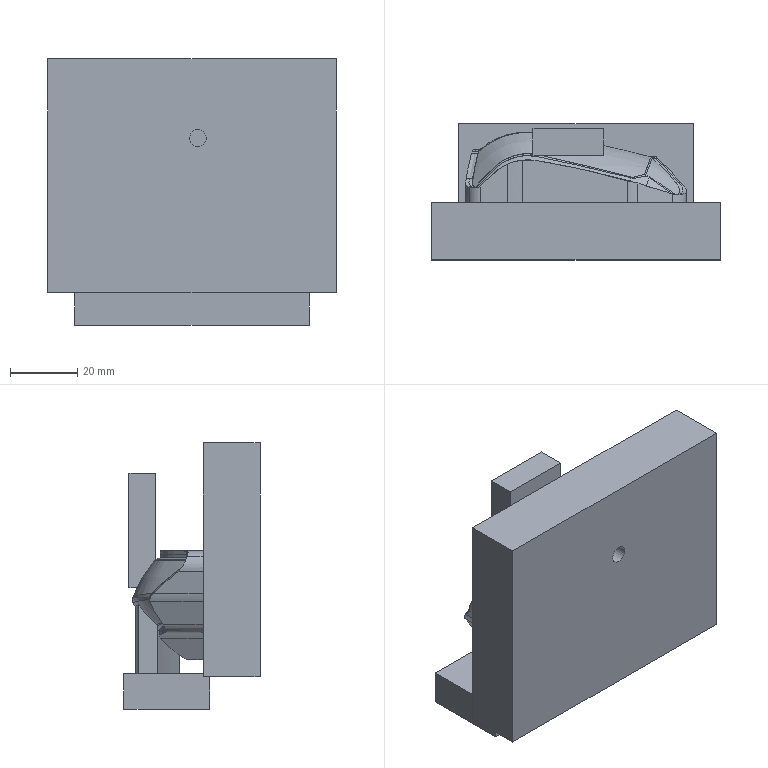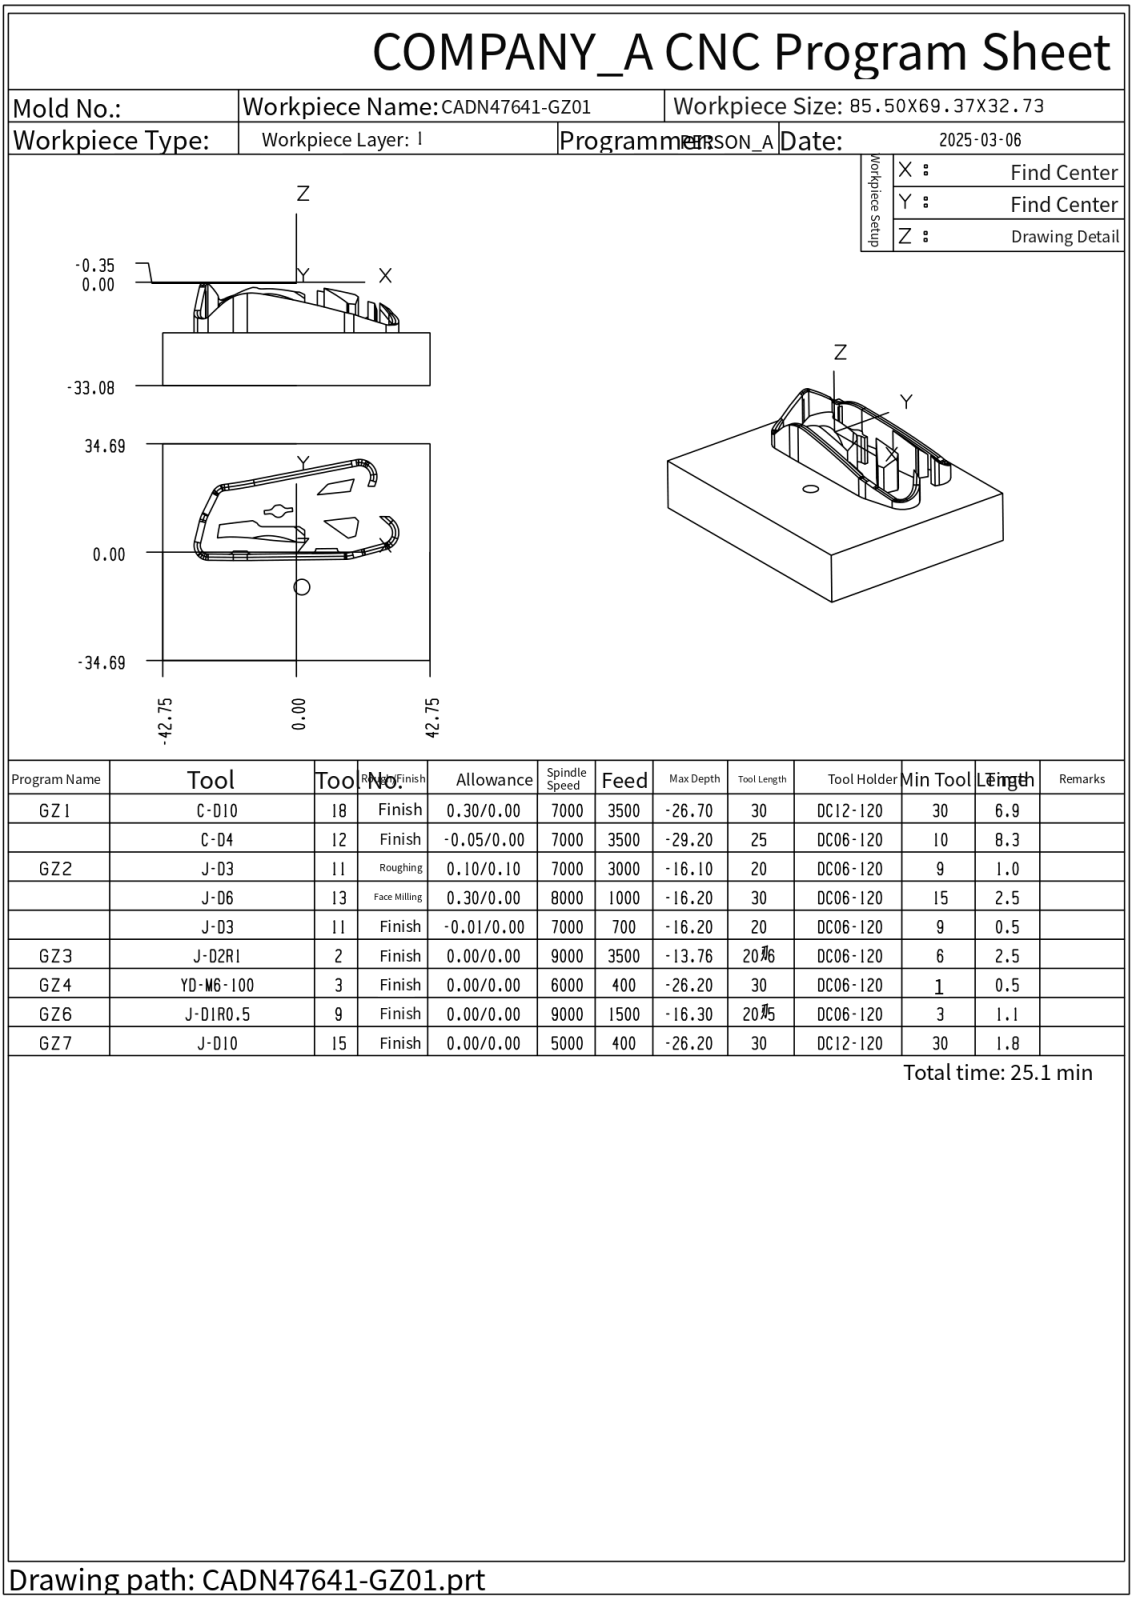NC program | NX | posted by the shop | part box 85.5 x 40.385 x 79 mm
Lines 20597 to 21518 of 71032:
20596 TOOL CALL 12 Z S7000
20597 CALL LBL101
20598 M3 M8
20599 M51
20600 CYCL DEF 32.0 TOLERANCE
20601 CYCL DEF 32.1 T0.012
20602 CYCL DEF 32.2 HSC-MODE:0
20603 L M126
20604 PLANE SPATIAL SPA-90. SPB+0.0 SPC+180. TURN FMAX SEQ-
20605 L X36.9624 Y34.3679 FMAX
20606 L Z102.5 FMAX
20607 L Z13.3944 FMAX
20608 L Z12.3944 F3500.
20609 CC X37.6151 Y33.3609
20610 C X36.5736 Y33.957 DR+
20611 CC X34.7509 Y35.
20612 C X34.7509 Y32.9 DR-
20613 L X-34.7509
20614 CC X-34.7509 Y35.
20615 C X-36.58 Y33.9681 DR-
20616 CC X-37.6251 Y33.3785
20617 C X-36.9662 Y34.3814 DR+
20618 L Z13.3944
20619 L Z102.5 FMAX
20620 L X36.9624 Y34.3679 FMAX
20621 L Z13.0966 FMAX
20622 L Z12.0966
20623 CC X37.6151 Y33.3609
20624 C X36.5736 Y33.957 DR+
20625 CC X34.7509 Y35.
20626 C X34.7509 Y32.9 DR-
20627 L X-34.7509
20628 CC X-34.7509 Y35.
20629 C X-36.58 Y33.9681 DR-
20630 CC X-37.6251 Y33.3785
20631 C X-36.9662 Y34.3814 DR+
20632 L Z13.0966
20633 L Z102.5 FMAX
20634 L X36.9624 Y34.3679 FMAX
20635 L Z12.7987 FMAX
20636 L Z11.7987
20637 CC X37.6151 Y33.361
20638 C X36.5736 Y33.957 DR+
20639 CC X34.7509 Y35.
20640 C X34.7509 Y32.9 DR-
20641 L X-34.7509
20642 CC X-34.7509 Y35.
20643 C X-36.5762 Y33.9615 DR-
20644 CC X-37.6192 Y33.3681
20645 C X-36.9639 Y34.3734 DR+
20646 L Z12.7987
20647 L Z102.5 FMAX
20648 L X36.9513 Y34.3304 FMAX
20649 L Z12.5008 FMAX
20650 L Z11.5008
20651 CC X37.5868 Y33.3125
20652 C X36.5556 Y33.9261 DR+
20653 CC X34.7509 Y35.
20654 C X34.7509 Y32.9 DR-
20655 L X-34.7509
20656 CC X-34.7509 Y35.
20657 C X-36.5499 Y33.9166 DR-
20658 CC X-37.5779 Y33.2975
20659 C X-36.9477 Y34.3187 DR+
20660 L Z12.5008
20661 L Z102.5 FMAX
20662 L X36.9411 Y34.2977 FMAX
20663 L Z12.2029 FMAX
20664 L Z11.2029
20665 CC X37.5614 Y33.2704
20666 C X36.5394 Y33.8993 DR+
20667 CC X34.7509 Y35.
20668 C X34.7509 Y32.9 DR-
20669 L X-34.7509
20670 CC X-34.7509 Y35.
20671 C X-36.5208 Y33.8697 DR-
20672 CC X-37.5321 Y33.2237
20673 C X-36.9291 Y34.2612 DR+
20674 L Z12.2029
20675 L Z102.5 FMAX
20676 L X36.9411 Y34.2977 FMAX
20677 L Z11.9051 FMAX
20678 L Z10.9051
20679 CC X37.5614 Y33.2704
20680 C X36.5394 Y33.8994 DR+
20681 CC X34.7509 Y35.
20682 C X34.7509 Y32.9 DR-
20683 L X-34.7509
20684 CC X-34.7509 Y35.
20685 C X-36.5208 Y33.8696 DR-
20686 CC X-37.5321 Y33.2237
20687 C X-36.9291 Y34.2612 DR+
20688 L Z11.9051
20689 L Z102.5 FMAX
20690 L X36.9411 Y34.2977 FMAX
20691 L Z11.6072 FMAX
20692 L Z10.6072
20693 CC X37.5614 Y33.2704
20694 C X36.5394 Y33.8994 DR+
20695 CC X34.7509 Y35.
20696 C X34.7509 Y32.9 DR-
20697 L X-34.7509
20698 CC X-34.7509 Y35.
20699 C X-36.5208 Y33.8696 DR-
20700 CC X-37.5321 Y33.2237
20701 C X-36.929 Y34.2612 DR+
20702 L Z11.6072
20703 L Z102.5 FMAX
20704 L X36.9411 Y34.2977 FMAX
20705 L Z11.3093 FMAX
20706 L Z10.3093
20707 CC X37.5614 Y33.2704
20708 C X36.5394 Y33.8994 DR+
20709 CC X34.7509 Y35.
20710 C X34.7509 Y32.9 DR-
20711 L X-34.7509
20712 CC X-34.7509 Y35.
20713 C X-36.5172 Y33.8641 DR-
20714 CC X-37.5265 Y33.215
20715 C X-36.9267 Y34.2543 DR+
20716 L Z11.3093
20717 L Z102.5 FMAX
20718 L X36.9411 Y34.2977 FMAX
20719 L Z11.0114 FMAX
20720 L Z10.0114
20721 CC X37.5614 Y33.2704
20722 C X36.5394 Y33.8994 DR+
20723 CC X34.7509 Y35.
20724 C X34.7509 Y32.9 DR-
20725 L X-34.7509
20726 CC X-34.7509 Y35.
20727 C X-36.5172 Y33.8641 DR-
20728 CC X-37.5265 Y33.215
20729 C X-36.9267 Y34.2544 DR+
20730 L Z11.0114
20731 L Z102.5 FMAX
20732 L X36.9411 Y34.2977 FMAX
20733 L Z10.7135 FMAX
20734 L Z9.7135
20735 CC X37.5614 Y33.2704
20736 C X36.5394 Y33.8994 DR+
20737 CC X34.7509 Y35.
20738 C X34.7509 Y32.9 DR-
20739 L X-34.7509
20740 CC X-34.7509 Y35.
20741 C X-36.5173 Y33.8642 DR-
20742 CC X-37.5266 Y33.2151
20743 C X-36.9268 Y34.2544 DR+
20744 L Z10.7135
20745 L Z102.5 FMAX
20746 L X36.9411 Y34.2977 FMAX
20747 L Z10.4157 FMAX
20748 L Z9.4157
20749 CC X37.5614 Y33.2704
20750 C X36.5394 Y33.8994 DR+
20751 CC X34.7509 Y35.
20752 C X34.7509 Y32.9 DR-
20753 L X-34.7509
20754 CC X-34.7509 Y35.
20755 C X-36.5173 Y33.8642 DR-
20756 CC X-37.5266 Y33.2152
20757 C X-36.9268 Y34.2545 DR+
20758 L Z10.4157
20759 L Z102.5 FMAX
20760 L X36.9411 Y34.2977 FMAX
20761 L Z10.1178 FMAX
20762 L Z9.1178
20763 CC X37.5614 Y33.2704
20764 C X36.5394 Y33.8994 DR+
20765 CC X34.7509 Y35.
20766 C X34.7509 Y32.9 DR-
20767 L X-34.7509
20768 CC X-34.7509 Y35.
20769 C X-36.5173 Y33.8643 DR-
20770 CC X-37.5267 Y33.2153
20771 C X-36.9268 Y34.2546 DR+
20772 L Z10.1178
20773 L Z102.5 FMAX
20774 L X36.9411 Y34.2977 FMAX
20775 L Z9.8199 FMAX
20776 L Z8.8199
20777 CC X37.5614 Y33.2704
20778 C X36.5394 Y33.8994 DR+
20779 CC X34.7509 Y35.
20780 C X34.7509 Y32.9 DR-
20781 L X-34.7509
20782 CC X-34.7509 Y35.
20783 C X-36.5174 Y33.8643 DR-
20784 CC X-37.5268 Y33.2154
20785 C X-36.9268 Y34.2546 DR+
20786 L Z9.8199
20787 L Z102.5 FMAX
20788 L X36.9411 Y34.2977 FMAX
20789 L Z9.522 FMAX
20790 L Z8.522
20791 CC X37.5614 Y33.2704
20792 C X36.5394 Y33.8994 DR+
20793 CC X34.7509 Y35.
20794 C X34.7509 Y32.9 DR-
20795 L X-34.7509
20796 CC X-34.7509 Y35.
20797 C X-36.5174 Y33.8644 DR-
20798 CC X-37.5268 Y33.2155
20799 C X-36.9268 Y34.2547 DR+
20800 L Z9.522
20801 L Z102.5 FMAX
20802 L X-18.6141 Y27.2829 FMAX
20803 L Z9.2242 FMAX
20804 L Z8.2242
20805 CC X-18.8159 Y26.1
20806 C X-18.8159 Y27.3 DR+
20807 L X-24.6183
20808 CC X-21.3134 Y27.7121
20809 C X-24.3883 Y28.9917 DR-
20810 L X-23.938 Y29.8719
20811 L X-23.8774 Y30.1
20812 L X-18.745
20813 CC X-18.745 Y28.9
20814 C X-18.5451 Y30.0832 DR-
20815 L Z9.2242
20816 L Z102.5 FMAX
20817 L X36.9411 Y34.2977 FMAX
20818 L Z9.2242 FMAX
20819 L Z8.2242
20820 CC X37.5614 Y33.2704
20821 C X36.5394 Y33.8994 DR+
20822 CC X34.7509 Y35.
20823 C X34.7509 Y32.9 DR-
20824 L X-34.7509
20825 CC X-34.7509 Y35.
20826 C X-36.5174 Y33.8644 DR-
20827 CC X-37.5269 Y33.2155
20828 C X-36.9269 Y34.2548 DR+
20829 L Z9.2242
20830 L Z102.5 FMAX
20831 L X36.9411 Y34.2977 FMAX
20832 L Z8.9263 FMAX
20833 L Z7.9263
20834 CC X37.5614 Y33.2705
20835 C X36.5394 Y33.8994 DR+
20836 CC X34.7509 Y35.
20837 C X34.7509 Y32.9 DR-
20838 L X-34.7509
20839 CC X-34.7509 Y35.
20840 C X-36.5175 Y33.8645 DR-
20841 CC X-37.5269 Y33.2156
20842 C X-36.9269 Y34.2548 DR+
20843 L Z8.9263
20844 L Z102.5 FMAX
20845 L X-24.3208 Y29.5463 FMAX
20846 L Z8.9263 FMAX
20847 L Z7.9263
20848 CC X-23.8929 Y30.6675
20849 C X-23.0586 Y29.805 DR+
20850 CC X-20.8283 Y27.4998
20851 C X-18.7898 Y29.9762 DR-
20852 CC X-20.2187 Y28.2403
20853 C X-19.1286 Y26.2739 DR-
20854 CC X-21.1131 Y29.8537
20855 C X-21.8613 Y25.8296 DR-
20856 CC X-21.4343 Y28.1262
20857 C X-23.0586 Y29.805 DR-
20858 CC X-23.8929 Y30.6675
20859 C X-23.0305 Y31.5019 DR+
20860 L Z8.9263
20861 L Z102.5 FMAX
20862 L X36.9411 Y34.2977 FMAX
20863 L Z8.6284 FMAX
20864 L Z7.6284
20865 CC X37.5614 Y33.2705
20866 C X36.5394 Y33.8994 DR+
20867 CC X34.7509 Y35.
20868 C X34.7509 Y32.9 DR-
20869 L X-34.7509
20870 CC X-34.7509 Y35.
20871 C X-36.5175 Y33.8646 DR-
20872 CC X-37.527 Y33.2157
20873 C X-36.9269 Y34.2549 DR+
20874 L Z8.6284
20875 L Z102.5 FMAX
20876 L X-20.4613 Y32.9 FMAX
20877 L Z8.1284 FMAX
20878 L Z7.6284
20879 L Y30.9706
20880 CC X-20.3237 Y27.3267
20881 C X-19.6546 Y30.9113 DR-
20882 CC X-20.5585 Y27.4379
20883 C X-17.6788 Y29.5801 DR-
20884 CC X-19.677 Y28.1643
20885 C X-18.5269 Y26.0023 DR-
20886 CC X-21.9205 Y32.1497
20887 C X-21.9101 Y25.1278 DR-
20888 CC X-21.9468 Y27.7207
20889 C X-24.4475 Y28.4067 DR-
20890 CC X-21.9276 Y27.8973
20891 C X-23.29 Y30.0776 DR-
20892 CC X-20.2499 Y25.3746
20893 C X-20.4613 Y30.9706 DR-
20894 CC X-20.5066 Y32.1698
20895 C X-19.3074 Y32.2151 DR+
20896 L Z8.6284
20897 L Z102.5 FMAX
20898 L X36.9408 Y34.2969 FMAX
20899 L Z8.3305 FMAX
20900 L Z7.3305
20901 CC X37.5608 Y33.2694
20902 C X36.539 Y33.8987 DR+
20903 CC X34.7509 Y35.
20904 C X34.7509 Y32.9 DR-
20905 L X-34.7509
20906 CC X-34.7509 Y35.
20907 C X-36.5175 Y33.8646 DR-
20908 CC X-37.527 Y33.2158
20909 C X-36.9269 Y34.255 DR+
20910 L Z8.3305
20911 L Z102.5 FMAX
20912 L X-19.1814 Y32.9 FMAX
20913 L Z7.8305 FMAX
20914 L Z7.3305
20915 L Y30.8717
20916 L X-19.0908 Y30.8541
20917 CC X-19.71 Y27.9787
20918 C X-17.8583 Y30.264 DR-
20919 CC X-19.4664 Y27.747
20920 C X-16.5644 Y28.4537 DR-
20921 CC X-18.9477 Y28.0463
20922 C X-17.6811 Y25.9867 DR-
20923 CC X-20.3906 Y30.2314
20924 C X-19.4596 Y25.2824 DR-
20925 CC X-18.7887 Y21.7159
20926 C X-20.2031 Y25.058 DR+
20927 CC X-22.0754 Y29.4817
20928 C X-22.7559 Y24.7266 DR-
20929 CC X-22.4253 Y27.2895
20930 C X-24.9385 Y27.8905 DR-
20931 CC X-22.5125 Y27.5713
20932 C X-24.2243 Y29.3197 DR-
20933 CC X-20.2499 Y25.3746
20934 C X-23.4112 Y29.997 DR-
20935 CC X-21.9276 Y27.8973
20936 C X-23.29 Y30.0776 DR-
20937 CC X-20.2499 Y25.3746
20938 C X-19.1814 Y30.8717 DR-
20939 CC X-18.9524 Y32.0497
20940 C X-17.7745 Y31.8207 DR+
20941 L Z8.3305
20942 L Z102.5 FMAX
20943 L X36.9411 Y34.2977 FMAX
20944 L Z8.0327 FMAX
20945 L Z7.0327
20946 CC X37.5614 Y33.2705
20947 C X36.5394 Y33.8994 DR+
20948 CC X34.7509 Y35.
20949 C X34.7509 Y32.9 DR-
20950 L X-34.7509
20951 CC X-34.7509 Y35.
20952 C X-36.5197 Y33.8679 DR-
20953 CC X-37.5304 Y33.221
20954 C X-36.9283 Y34.259 DR+
20955 L Z8.0327
20956 L Z102.5 FMAX
20957 L X-19.1814 Y32.9 FMAX
20958 L Z7.5327 FMAX
20959 L Z7.0327
20960 L Y30.8717
20961 L X-18.4538 Y30.7303
20962 CC X-18.9259 Y28.1169
20963 C X-17.3992 Y30.2899 DR-
20964 CC X-19.5469 Y26.6047
20965 C X-16.3645 Y29.4448 DR-
20966 CC X-18.1174 Y27.8804
20967 C X-16.8627 Y25.894 DR-
20968 CC X-19.5211 Y30.1026
20969 C X-19.3727 Y25.1269 DR-
20970 L X-19.6546 Y25.0952
20971 CC X-19.531 Y24.1434
20972 C X-20.0756 Y24.9337 DR+
20973 L X-20.2185 Y24.8398
20974 CC X-22.2304 Y28.1972
20975 C X-23.0379 Y24.3673 DR-
20976 L X-23.2451 Y24.411
20977 CC X-22.7061 Y26.9633
20978 C X-25.3133 Y27.0457 DR-
20979 CC X-22.9822 Y27.1637
20980 C X-24.9349 Y28.4423 DR-
20981 CC X-20.2499 Y25.3746
20982 C X-24.3108 Y29.2307 DR-
20983 L X-24.2243 Y29.3197
20984 CC X-20.2499 Y25.3746
20985 C X-23.4112 Y29.997 DR-
20986 CC X-21.9276 Y27.8973
20987 C X-23.29 Y30.0776 DR-
20988 CC X-20.2499 Y25.3746
20989 C X-19.1814 Y30.8717 DR-
20990 CC X-18.9524 Y32.0497
20991 C X-17.7745 Y31.8207 DR+
20992 L Z8.0327
20993 L Z102.5 FMAX
20994 L X36.9411 Y34.2977 FMAX
20995 L Z7.7348 FMAX
20996 L Z6.7348
20997 CC X37.5614 Y33.2705
20998 C X36.5394 Y33.8994 DR+
20999 CC X34.7509 Y35.
21000 C X34.7509 Y32.9 DR-
21001 L X-34.7509
21002 CC X-34.7509 Y35.
21003 C X-36.5196 Y33.8679 DR-
21004 CC X-37.5303 Y33.2209
21005 C X-36.9283 Y34.259 DR+
21006 L Z7.7348
21007 L Z102.5 FMAX
21008 L X-19.1814 Y32.9 FMAX
21009 L Z7.2348 FMAX
21010 L Z6.7348
21011 L Y30.8717
21012 L X-17.6635 Y30.5767
21013 CC X-18.2042 Y27.8542
21014 C X-16.6344 Y30.1433 DR-
21015 CC X-18.4639 Y26.6336
21016 C X-15.5016 Y29.2584 DR-
21017 CC X-17.242 Y27.7162
21018 C X-16.1081 Y25.6861 DR-
21019 CC X-18.7961 Y30.4986
21020 C X-18.8088 Y24.9863 DR-
21021 L X-19.0908 Y24.9972
21022 CC X-19.1896 Y21.8556
21023 C X-19.6546 Y24.9641 DR+
21024 CC X-19.5704 Y24.3133
21025 C X-20.0184 Y24.7929 DR+
21026 CC X-22.1412 Y27.0882
21027 C X-21.9101 Y23.9703 DR-
21028 CC X-22.2495 Y29.4894
21029 C X-23.6017 Y24.1277 DR-
21030 CC X-22.9769 Y26.5808
21031 C X-25.4203 Y25.9193 DR-
21032 CC X-23.1143 Y26.7129
21033 C X-25.3459 Y27.6964 DR-
21034 CC X-20.2499 Y25.3746
21035 C X-23.4112 Y29.997 DR-
21036 CC X-21.9276 Y27.8973
21037 C X-23.29 Y30.0776 DR-
21038 CC X-20.2499 Y25.3746
21039 C X-19.1814 Y30.8717 DR-
21040 CC X-18.9524 Y32.0497
21041 C X-17.7745 Y31.8207 DR+
21042 L Z7.7348
21043 L Z102.5 FMAX
21044 L X36.9411 Y34.2977 FMAX
21045 L Z7.4369 FMAX
21046 L Z6.4369
21047 CC X37.5614 Y33.2705
21048 C X36.5394 Y33.8994 DR+
21049 CC X34.7509 Y35.
21050 C X34.7509 Y32.9 DR-
21051 L X-34.7509
21052 CC X-34.7509 Y35.
21053 C X-36.5196 Y33.8679 DR-
21054 CC X-37.5303 Y33.2209
21055 C X-36.9283 Y34.259 DR+
21056 L Z7.4369
21057 L Z102.5 FMAX
21058 L X-19.1814 Y32.9 FMAX
21059 L Z6.9369 FMAX
21060 L Z6.4369
21061 L Y30.8717
21062 L X-16.8385 Y30.4163
21063 CC X-17.6049 Y26.986
21064 C X-15.7076 Y29.9448 DR-
21065 CC X-17.5522 Y26.1956
21066 C X-14.7538 Y29.2985 DR-
21067 CC X-16.2943 Y27.5455
21068 C X-15.4256 Y25.3796 DR-
21069 CC X-18.5233 Y33.056
21070 C X-17.6811 Y24.8211 DR-
21071 CC X-18.0731 Y32.5491
21072 C X-18.8923 Y24.8546 DR-
21073 CC X-19.1897 Y22.0614
21074 C X-19.6548 Y24.8317 DR+
21075 CC X-19.5756 Y24.3601
21076 C X-19.937 Y24.6732 DR+
21077 CC X-22.1627 Y26.6011
21078 C X-22.2759 Y23.6587 DR-
21079 CC X-21.7153 Y38.2392
21080 C X-23.3198 Y23.7364 DR-
21081 CC X-23.0742 Y26.3604
21082 C X-25.7075 Y26.469 DR-
21083 CC X-23.8598 Y26.3928
21084 C X-25.6396 Y26.8948 DR-
21085 CC X-20.2499 Y25.3746
21086 C X-23.4112 Y29.997 DR-
21087 CC X-21.9276 Y27.8973
21088 C X-23.29 Y30.0776 DR-
21089 CC X-20.2499 Y25.3746
21090 C X-19.1814 Y30.8717 DR-
21091 CC X-18.9524 Y32.0497
21092 C X-17.7745 Y31.8207 DR+
21093 L Z7.4369
21094 L Z102.5 FMAX
21095 L X36.9411 Y34.2977 FMAX
21096 L Z7.139 FMAX
21097 L Z6.139
21098 CC X37.5614 Y33.2705
21099 C X36.5394 Y33.8994 DR+
21100 CC X34.7509 Y35.
21101 C X34.7509 Y32.9 DR-
21102 L X-34.7509
21103 CC X-34.7509 Y35.
21104 C X-36.5196 Y33.8678 DR-
21105 CC X-37.5303 Y33.2209
21106 C X-36.9283 Y34.2589 DR+
21107 L Z7.139
21108 L Z102.5 FMAX
21109 L X-19.1814 Y32.9 FMAX
21110 L Z6.639 FMAX
21111 L Z6.139
21112 L Y30.8717
21113 L X-15.921 Y30.238
21114 CC X-16.6418 Y26.8208
21115 C X-14.8617 Y29.8255 DR-
21116 CC X-16.9521 Y25.3303
21117 C X-13.7113 Y29.0818 DR-
21118 CC X-15.2108 Y27.3459
21119 C X-14.4474 Y25.1829 DR-
21120 CC X-17.8878 Y34.9305
21121 C X-16.8353 Y24.6473 DR-
21122 CC X-17.3482 Y33.0706
21123 C X-18.245 Y24.6794 DR-
21124 CC X-19.5653 Y10.5716
21125 C X-19.3727 Y24.7398 DR+
21126 CC X-19.365 Y23.8517
21127 C X-19.7956 Y24.6284 DR+
21128 CC X-22.6155 Y26.6846
21129 C X-20.2693 Y24.101 DR-
21130 CC X-22.1519 Y26.1741
21131 C X-22.4189 Y23.3865 DR-
21132 CC X-23.4048 Y13.0898
21133 C X-23.2453 Y23.4324 DR+
21134 CC X-23.2048 Y26.0575
21135 C X-25.7348 Y25.3561 DR-
21136 CC X-23.4844 Y25.9199
21137 C X-25.7768 Y26.2768 DR-
21138 CC X-20.2499 Y25.3746
21139 C X-23.4112 Y29.997 DR-
21140 CC X-21.9276 Y27.8973
21141 C X-23.29 Y30.0776 DR-
21142 CC X-20.2499 Y25.3746
21143 C X-19.1814 Y30.8717 DR-
21144 CC X-18.9524 Y32.0497
21145 C X-17.7745 Y31.8207 DR+
21146 L Z7.139
21147 L Z102.5 FMAX
21148 L X36.9411 Y34.2977 FMAX
21149 L Z6.8412 FMAX
21150 L Z5.8412
21151 CC X37.5614 Y33.2705
21152 C X36.5394 Y33.8994 DR+
21153 CC X34.7509 Y35.
21154 C X34.7509 Y32.9 DR-
21155 L X-34.7509
21156 CC X-34.7509 Y35.
21157 C X-36.5196 Y33.8678 DR-
21158 CC X-37.5302 Y33.2208
21159 C X-36.9283 Y34.2589 DR+
21160 L Z6.8412
21161 L Z102.5 FMAX
21162 L X-19.1814 Y32.9 FMAX
21163 L Z6.3412 FMAX
21164 L Z5.8412
21165 L Y30.8717
21166 L X-14.8936 Y30.0382
21167 CC X-15.7635 Y26.0739
21168 C X-13.734 Y29.5887 DR-
21169 CC X-15.4847 Y25.6388
21170 C X-13.0904 Y29.2352 DR-
21171 L X-11.8769 Y30.8686
21172 L X-13.0904 Y29.2352
21173 CC X-15.4847 Y25.6388
21174 C X-12.5449 Y28.8049 DR-
21175 CC X-14.0941 Y27.1364
21176 C X-13.3638 Y24.9798 DR-
21177 CC X-16.554 Y34.4
21178 C X-15.4901 Y24.5113 DR-
21179 CC X-16.4706 Y31.3942
21180 C X-16.9308 Y24.4571 DR-
21181 L X-17.3992 Y24.4882
21182 L X-18.8088 Y24.5918
21183 L X-19.2047 Y24.6194
21184 CC X-19.2746 Y23.6175
21185 C X-19.7197 Y24.5179 DR+
21186 CC X-22.1442 Y25.8987
21187 C X-22.4879 Y23.1298 DR-
21188 CC X-22.8233 Y20.4282
21189 C X-23.0496 Y23.1411 DR+
21190 CC X-23.271 Y25.7952
21191 C X-25.4257 Y24.2297 DR-
21192 CC X-23.5748 Y25.5454
21193 C X-25.8439 Y25.6349 DR-
21194 CC X-20.2499 Y25.3746
21195 C X-23.4112 Y29.997 DR-
21196 CC X-21.9276 Y27.8973
21197 C X-23.29 Y30.0776 DR-
21198 CC X-20.2499 Y25.3746
21199 C X-19.1814 Y30.8717 DR-
21200 CC X-18.9524 Y32.0497
21201 C X-17.7745 Y31.8207 DR+
21202 L Z6.8412
21203 L Z102.5 FMAX
21204 L X36.9411 Y34.2977 FMAX
21205 L Z6.5433 FMAX
21206 L Z5.5433
21207 CC X37.5614 Y33.2705
21208 C X36.5394 Y33.8994 DR+
21209 CC X34.7509 Y35.
21210 C X34.7509 Y32.9 DR-
21211 L X-34.7509
21212 CC X-34.7509 Y35.
21213 C X-36.5196 Y33.8678 DR-
21214 CC X-37.5302 Y33.2208
21215 C X-36.9283 Y34.2589 DR+
21216 L Z6.5433
21217 L Z102.5 FMAX
21218 L X-19.1814 Y32.9 FMAX
21219 L Z6.0433 FMAX
21220 L Z5.5433
21221 L Y30.8717
21222 L X-13.7911 Y29.824
21223 CC X-14.3705 Y26.7903
21224 C X-12.8882 Y29.4998 DR-
21225 CC X-14.709 Y25.0085
21226 C X-11.409 Y28.5578 DR-
21227 CC X-12.9382 Y26.913
21228 C X-11.9787 Y24.8825 DR-
21229 CC X-14.2114 Y29.607
21230 C X-13.734 Y24.4033 DR-
21231 CC X-15.5184 Y34.7673
21232 C X-16.2886 Y24.2791 DR-
21233 L X-19.0908 Y24.4848
21234 L X-19.2384 Y24.4907
21235 CC X-19.2901 Y23.7112
21236 C X-19.6398 Y24.4098 DR+
21237 CC X-22.1553 Y25.6288
21238 C X-21.6282 Y22.8836 DR-
21239 CC X-22.1804 Y27.5486
21240 C X-22.7559 Y22.8865 DR-
21241 CC X-23.2983 Y25.5474
21242 C X-25.2571 Y23.6665 DR-
21243 CC X-23.5952 Y25.1822
21244 C X-25.8395 Y25.0336 DR-
21245 CC X-20.2499 Y25.3746
21246 C X-23.4112 Y29.997 DR-
21247 CC X-21.9276 Y27.8973
21248 C X-23.29 Y30.0776 DR-
21249 CC X-20.2499 Y25.3746
21250 C X-19.1814 Y30.8717 DR-
21251 CC X-18.9524 Y32.0497
21252 C X-17.7745 Y31.8207 DR+
21253 L Z6.5433
21254 L X-10.1771 Y30.8833 Z6.2454 FMAX
21255 L Z5.2454
21256 CC X-10.3768 Y29.7
21257 C X-10.3768 Y30.9 DR+
21258 L X-10.5162
21259 CC X-12.6545 Y26.123
21260 C X-10.3847 Y30.839 DR-
21261 CC X-9.8643 Y31.9202
21262 C X-10.1911 Y30.7656 DR+
21263 L Z6.2454
21264 L Z102.5 FMAX
21265 L X36.9411 Y34.2977 FMAX
21266 L Z6.2454 FMAX
21267 L Z5.2454
21268 CC X37.5614 Y33.2705
21269 C X36.5394 Y33.8994 DR+
21270 CC X34.7509 Y35.
21271 C X34.7509 Y32.9 DR-
21272 L X-34.7509
21273 CC X-34.7509 Y35.
21274 C X-36.5196 Y33.8677 DR-
21275 CC X-37.5302 Y33.2207
21276 C X-36.9283 Y34.2588 DR+
21277 L Z6.2454
21278 L Z102.5 FMAX
21279 L X-10.5162 Y30.9 FMAX
21280 L Z6.2454 FMAX
21281 L Z5.2454
21282 L X-19.1814 Y30.8717
21283 L X-12.6853 Y29.609
21284 CC X-13.6106 Y25.4773
21285 C X-11.4785 Y29.1354 DR-
21286 CC X-12.6545 Y26.123
21287 C X-9.6534 Y27.3273 DR-
21288 CC X-11.8741 Y26.694
21289 C X-11.1966 Y24.4864 DR-
21290 L X-11.4785 Y24.3978
21291 CC X-14.3698 Y35.9693
21292 C X-15.1437 Y24.0672 DR-
21293 L X-19.1774 Y24.3645
21294 CC X-19.2397 Y23.5188
21295 C X-19.5514 Y24.3074 DR+
21296 CC X-22.2575 Y25.4343
21297 C X-20.7824 Y22.9011 DR-
21298 CC X-22.0963 Y25.3172
21299 C X-22.626 Y22.6184 DR-
21300 CC X-23.3197 Y25.2055
21301 C X-25.0114 Y23.1289 DR-
21302 CC X-23.5909 Y24.8279
21303 C X-25.7754 Y24.4643 DR-
21304 CC X-20.2499 Y25.3746
21305 C X-23.4112 Y29.997 DR-
21306 CC X-21.9276 Y27.8973
21307 C X-23.29 Y30.0776 DR-
21308 CC X-20.2499 Y25.3746
21309 C X-19.1814 Y30.8717 DR-
21310 CC X-18.9524 Y32.0497
21311 C X-17.7745 Y31.8207 DR+
21312 L Z6.2454
21313 L X-9.0647 Y30.8832 Z5.9475 FMAX
21314 L Z4.9475
21315 CC X-9.2646 Y29.7
21316 C X-9.2646 Y30.9 DR+
21317 L X-9.8499
21318 CC X-12.2136 Y26.1479
21319 C X-9.7613 Y30.8549 DR-
21320 CC X-13.0378 Y23.473
21321 C X-9.2887 Y30.6265 DR-
21322 CC X-8.7317 Y31.6893
21323 C X-9.0886 Y30.5436 DR+
21324 L Z5.9475
21325 L Z102.5 FMAX
21326 L X36.9411 Y34.2977 FMAX
21327 L Z5.9475 FMAX
21328 L Z4.9475
21329 CC X37.5614 Y33.2705
21330 C X36.5394 Y33.8994 DR+
21331 CC X34.7509 Y35.
21332 C X34.7509 Y32.9 DR-
21333 L X-34.7509
21334 CC X-34.7509 Y35.
21335 C X-36.5195 Y33.8677 DR-
21336 CC X-37.5302 Y33.2207
21337 C X-36.9282 Y34.2588 DR+
21338 L Z5.9475
21339 L Z102.5 FMAX
21340 L X-9.8499 Y30.9 FMAX
21341 L Z5.9475 FMAX
21342 L Z4.9475
21343 L X-19.1814 Y30.8717
21344 L X-11.5784 Y29.3939
21345 CC X-12.2137 Y26.1479
21346 C X-10.6327 Y29.0531 DR-
21347 CC X-13.0378 Y23.473
21348 C X-9.223 Y28.2027 DR-
21349 CC X-10.6941 Y26.4338
21350 C X-10.0347 Y24.2297 DR-
21351 CC X-13.0687 Y35.126
21352 C X-13.734 Y23.8348 DR-
21353 L X-19.1915 Y24.2388
21354 CC X-19.2411 Y23.568
21355 C X-19.4591 Y24.2044 DR+
21356 CC X-22.2366 Y25.1418
21357 C X-20.5004 Y22.7798 DR-
21358 CC X-22.0167 Y24.8427
21359 C X-22.5133 Y22.3311 DR-
21360 CC X-23.2803 Y24.8669
21361 C X-25.0114 Y22.8615 DR-
21362 CC X-23.5424 Y24.485
21363 C X-25.6569 Y23.9171 DR-
21364 CC X-20.2499 Y25.3746
21365 C X-23.4112 Y29.997 DR-
21366 CC X-21.9276 Y27.8973
21367 C X-23.29 Y30.0776 DR-
21368 CC X-20.2499 Y25.3746
21369 C X-19.1814 Y30.8717 DR-
21370 CC X-18.9524 Y32.0497
21371 C X-17.7745 Y31.8207 DR+
21372 L Z5.9475
21373 L Z102.5 FMAX
21374 L X36.9411 Y34.2977 FMAX
21375 L Z5.6497 FMAX
21376 L Z4.6497
21377 CC X37.5614 Y33.2705
21378 C X36.5394 Y33.8994 DR+
21379 CC X34.7509 Y35.
21380 C X34.7509 Y32.9 DR-
21381 L X-34.7509
21382 CC X-34.7509 Y35.
21383 C X-36.5195 Y33.8677 DR-
21384 CC X-37.5302 Y33.2207
21385 C X-36.9282 Y34.2588 DR+
21386 L Z5.6497
21387 L Z102.5 FMAX
21388 L X-19.1814 Y32.9 FMAX
21389 L Z5.1497 FMAX
21390 L Z4.6497
21391 L Y30.8717
21392 L X-10.5146 Y29.1871
21393 CC X-11.5174 Y24.5818
21394 C X-9.223 Y28.6988 DR-
21395 CC X-10.5574 Y25.3562
21396 C X-7.3795 Y27.0457 DR-
21397 CC X-9.5507 Y26.201
21398 C X-8.9225 Y23.9575 DR-
21399 CC X-11.6476 Y33.6886
21400 C X-12.3243 Y23.6059 DR-
21401 L X-12.6063 Y23.6152
21402 L X-13.734 Y23.7002
21403 L X-14.2979 Y23.7469
21404 L X-18.245 Y24.0422
21405 L X-19.0742 Y24.0993
21406 CC X-19.1672 Y22.7499
21407 C X-19.3652 Y24.0879 DR+
21408 CC X-22.1322 Y24.7919
21409 C X-20.5004 Y22.449 DR-
21410 CC X-21.9595 Y24.6323
21411 C X-22.391 Y22.042 DR-
21412 CC X-23.1934 Y24.6059
21413 C X-24.7295 Y22.4019 DR-
21414 CC X-23.4369 Y24.1803
21415 C X-25.5193 Y23.4754 DR-
21416 L X-25.5566 Y23.5861
21417 CC X-20.2499 Y25.3746
21418 C X-23.4112 Y29.997 DR-
21419 CC X-21.9276 Y27.8973
21420 C X-23.29 Y30.0776 DR-
21421 CC X-20.2499 Y25.3746
21422 C X-19.1814 Y30.8717 DR-
21423 CC X-18.9524 Y32.0497
21424 C X-17.7745 Y31.8207 DR+
21425 L Z5.6497
21426 L X-8.0484 Y30.8833 Z5.3518 FMAX
21427 L Z4.3518
21428 CC X-8.2481 Y29.7
21429 C X-8.2481 Y30.9 DR+
21430 L X-8.8539
21431 CC X-10.1092 Y25.2539
21432 C X-8.2658 Y30.7362 DR-
21433 CC X-7.8833 Y31.8737
21434 C X-8.0682 Y30.688 DR+
21435 L Z5.3518
21436 L Z102.5 FMAX
21437 L X-25.4595 Y28.0042 FMAX
21438 L Z5.3518 FMAX
21439 L Z4.3518
21440 CC X-25.9347 Y29.1061
21441 C X-24.9315 Y28.4476 DR+
21442 CC X-20.2499 Y25.3746
21443 C X-23.4112 Y29.997 DR-
21444 CC X-21.9275 Y27.8973
21445 C X-23.29 Y30.0776 DR-
21446 CC X-20.2499 Y25.3746
21447 C X-19.1814 Y30.8717 DR-
21448 L X-9.3319 Y28.9572
21449 CC X-10.1092 Y25.2539
21450 C X-8.3772 Y28.6182 DR-
21451 CC X-11.1229 Y22.1718
21452 C X-6.9559 Y27.8048 DR-
21453 CC X-8.33 Y25.9473
21454 C X-7.6771 Y23.7308 DR-
21455 CC X-10.3822 Y32.9131
21456 C X-11.1966 Y23.3753 DR-
21457 L X-17.6811 Y23.8731
21458 CC X-18.7591 Y7.9964
21459 C X-19.2576 Y23.9019 DR+
21460 CC X-21.9342 Y24.4218
21461 C X-20.7824 Y21.9504 DR-
21462 CC X-21.84 Y24.2197
21463 C X-22.273 Y21.7538 DR-
21464 CC X-23.0875 Y24.3465
21465 C X-24.4475 Y21.9937 DR-
21466 CC X-23.3431 Y23.8904
21467 C X-25.4285 Y23.2058 DR-
21468 L X-25.5566 Y23.5861
21469 CC X-20.2499 Y25.3746
21470 C X-25.1014 Y28.1716 DR-
21471 CC X-26.141 Y28.771
21472 C X-24.9497 Y28.9149 DR+
21473 L Z5.3518
21474 L Z102.5 FMAX
21475 L X36.9411 Y34.2977 FMAX
21476 L Z5.3518 FMAX
21477 L Z4.3518
21478 CC X37.5614 Y33.2705
21479 C X36.5394 Y33.8994 DR+
21480 CC X34.7509 Y35.
21481 C X34.7509 Y32.9 DR-
21482 L X-34.7509
21483 CC X-34.7509 Y35.
21484 C X-36.5192 Y33.8672 DR-
21485 CC X-37.5296 Y33.2198
21486 C X-36.928 Y34.2581 DR+
21487 L Z5.3518
21488 L Z102.5 FMAX
21489 L X-8.0475 Y30.8833 FMAX
21490 L Z5.0539 FMAX
21491 L Z4.0539
21492 CC X-8.2473 Y29.7
21493 C X-8.2473 Y30.9 DR+
21494 L X-8.8452
21495 L X-8.2609 Y30.7864
21496 CC X-8.032 Y31.9644
21497 C X-8.0621 Y30.7648 DR+
21498 L Z5.0539
21499 L Z102.5 FMAX
21500 L X-25.4662 Y27.9952 FMAX
21501 L Z5.0539 FMAX
21502 L Z4.0539
21503 CC X-25.9402 Y29.0976
21504 C X-24.936 Y28.4406 DR+
21505 CC X-20.2499 Y25.3746
21506 C X-23.4112 Y29.997 DR-
21507 CC X-21.9275 Y27.8973
21508 C X-23.29 Y30.0776 DR-
21509 CC X-20.2499 Y25.3746
21510 C X-19.1814 Y30.8717 DR-
21511 L X-8.1706 Y28.7314
21512 CC X-8.8605 Y25.2704
21513 C X-7.2495 Y28.4104 DR-
21514 CC X-9.3625 Y22.9871
21515 C X-5.6144 Y27.44 DR-
21516 CC X-7.0796 Y25.6992
21517 C X-6.3218 Y23.5537 DR-